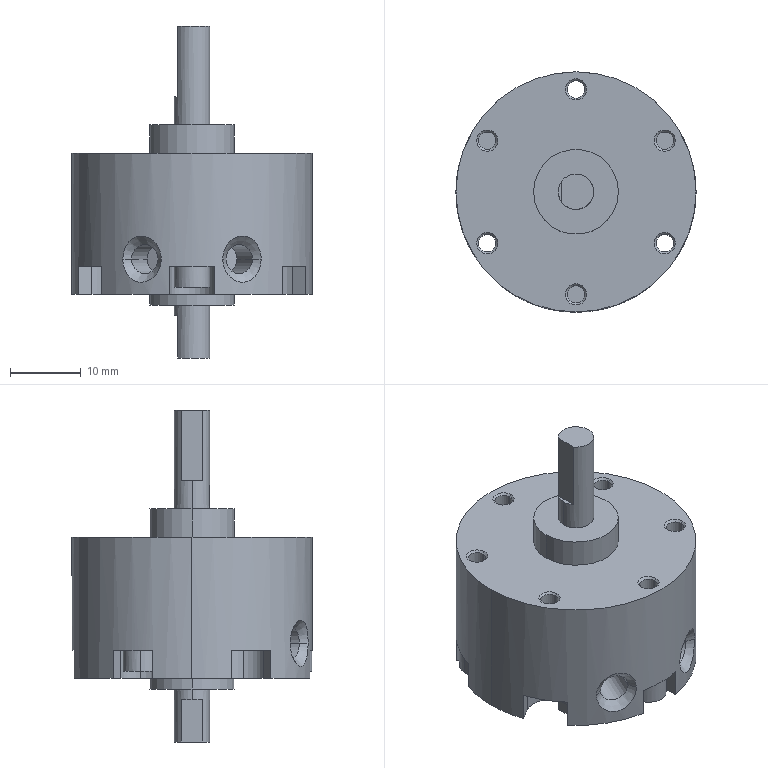Part | STEP file | CDRB2BW15-180S | 1 solid | 104 faces | box 34 x 34 x 47 mm | volume 18029 mm3 | cylinder 46 | plane 36 | cone 22 | commonest cylinder face diameters 2.459 x12 5 x10 6.5 x8 3.4 x6 4.134 x4 12 x4